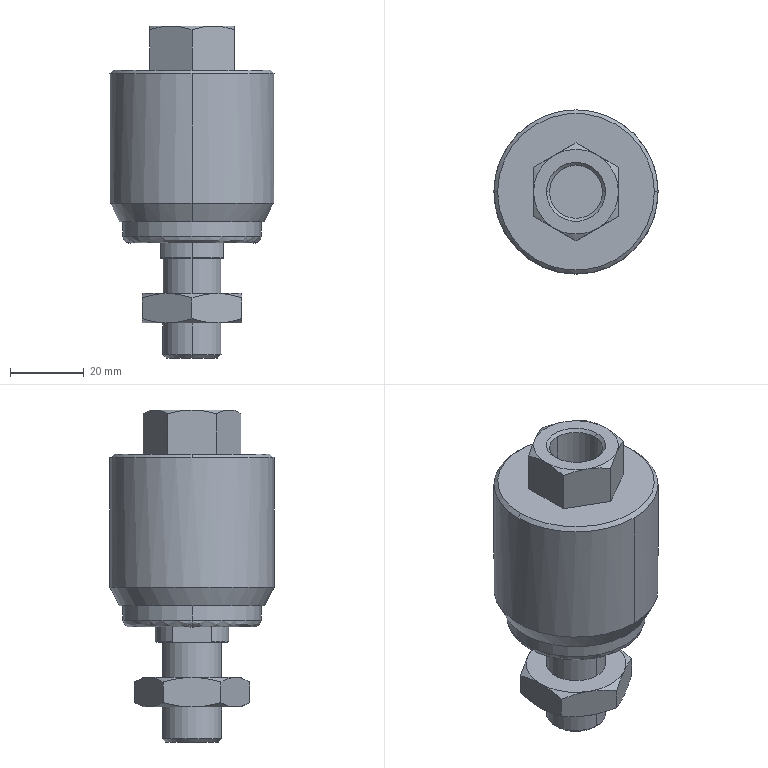Part | SolidWorks | features BaseBody 1 | 1 solid | 73 faces | box 44.5 x 44.5 x 90 mm | volume 81124 mm3 | cone 34 | plane 24 | cylinder 13 | spline 2 | commonest cylinder face diameters 16 x4 20 x3 14.376 x2 37.5 x2 44.5 x2